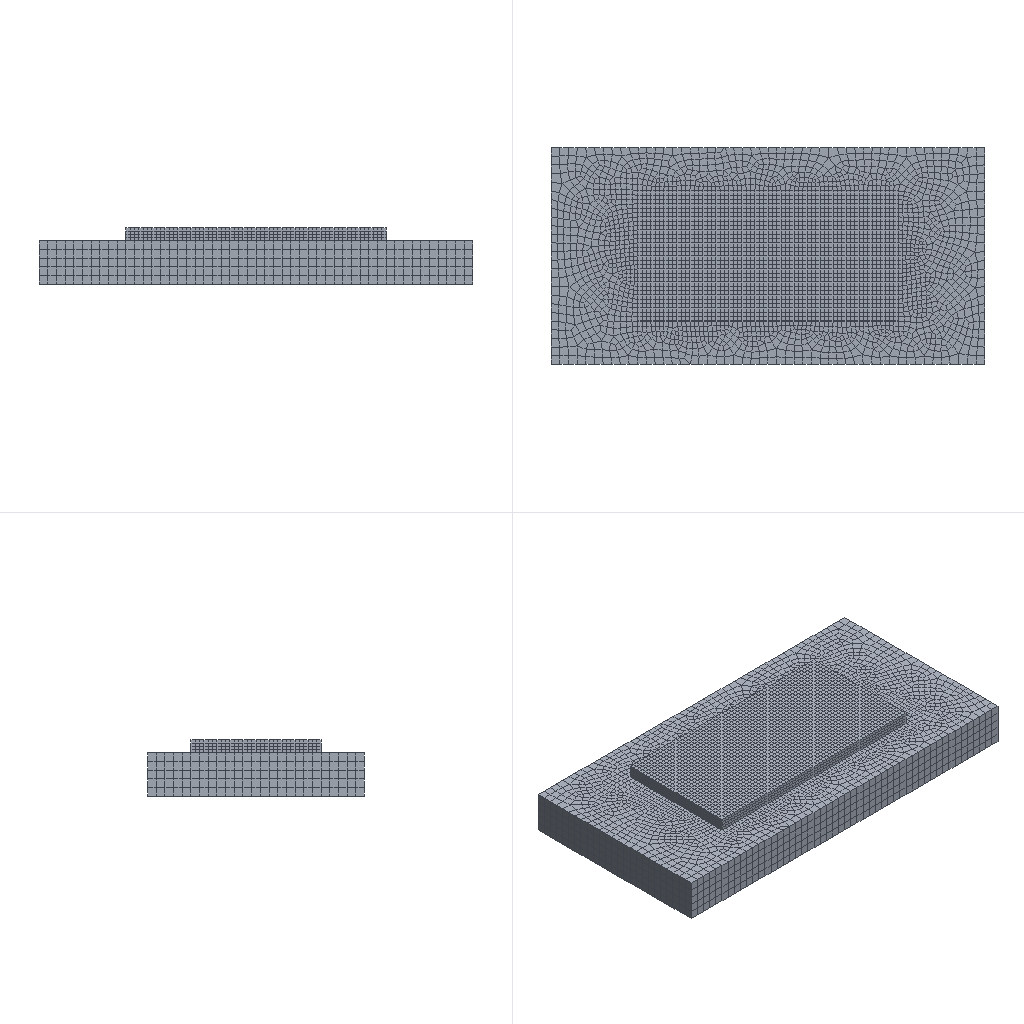Simulation study | abaqus
Set-up summary:
category,name,step,type,value,unit,region
solver,abaqus
solver,version,,,Abaqus/Standard 3DEXPERIENCE R2017x
units,not stated in the deck,,not stated
analysis,deck,,thermal,thermal
load_step,Step-1-del-all,Step-1-del-all,thermal
load_step,Step-add1,Step-add1,thermal
load_step,Step-add-l1,Step-add-l1,thermal
load_step,Step-add2,Step-add2,thermal
load_step,Step-add2-l2,Step-add2-l2,thermal
load_step,Step-add3,Step-add3,thermal
load_step,Step-add3-l3,Step-add3-l3,thermal
load_step,Step-add4,Step-add4,thermal
load_step,Step-add4-l4,Step-add4-l4,thermal
load_step,Step-add5,Step-add5,thermal
load_step,Step-add5-l5,Step-add5-l5,thermal
load_step,Step-stop1,Step-stop1,thermal
load_step,Step-add6,Step-add6,thermal
load_step,Step-add6-l6,Step-add6-l6,thermal
load_step,Step-add7,Step-add7,thermal
load_step,Step-add7-l7,Step-add7-l7,thermal
load_step,Step-add8,Step-add8,thermal
load_step,Step-add8-l8,Step-add8-l8,thermal
load_step,Step-add9,Step-add9,thermal
load_step,Step-add9-l9,Step-add9-l9,thermal
load_step,Step-add10,Step-add10,thermal
load_step,Step-add10-l10,Step-add10-l10,thermal
load_step,Step-stop2,Step-stop2,thermal
load_step,requested,,,23
mesh,nodes,,,29512
mesh,elements,,,25110
element_type,DC3D8,,solid,25110
load,load commands in deck,,count,21
bc,support commands in deck,,count,2
material,ADD,,in results
material,MATERIAL-1,,in results
check,setup vs results,,match,"per instance, exact: element labels, types and connectivity; labels of the nodes the elements use; coordinates of those nodes at SINGLE_PRECISION in 1 of 1 instance(s)"
Abaqus input file, long lists of numbers shortened:
*Heading
** Job name: Job-1 Model name: Model-1
** Generated by: Abaqus/CAE 2017
*Preprint, echo=NO, model=NO, history=NO, contact=NO
**
** PARTS
**
*Part, name=Part-1
*Node
      1,          10.,         -17.,         5.75
      2,          10.,         -17.,           5.
** (29510 more lines like these left out)
*Element, type=DC3D8
  1,   294,  2297, 12531,  1707,     1,    45,  1589,   164
  2,  2297,   300,  2002, 12531,    45,     2,    46,  1589
** (25108 more lines like these left out)
*Nset, nset=Set-1
     2,     3,     5,     6,    10,    11,    25,    26,    27,    28,    35,    36,    37,    38,    39,    40
    41,    42,    43,    44,    46,    47,    48,    49,    50,    51,    52,    53,    54,    55,    56,    57
** (1370 more lines like these left out)
*Elset, elset=Set-1, generate
  7201,  25110,      1
*Nset, nset=Set-4
     1,     2,     3,     4,     5,     6,     7,     8,     9,    10,    11,    12,    13,    14,    15,    16
    17,    18,    19,    20,    21,    22,    23,    24,    25,    26,    27,    28,    29,    30,    31,    32
** (589 more lines like these left out)
*Elset, elset=Set-4, generate
    1,  7200,     1
** Section: add
*Solid Section, elset=Set-4, material=add
,
** Section: steel
*Solid Section, elset=Set-1, material=Material-1
,
*End Part
**
**
** ASSEMBLY
**
*Assembly, name=Assembly
**
*Instance, name=Part-1-1, part=Part-1
*End Instance
**
*Nset, nset=Set-1, instance=Part-1-1
     1,     2,     3,     4,     5,     6,     7,     8,     9,    10,    11,    12,    13,    14,    15,    16
    17,    18,    19,    20,    21,    22,    23,    24,    25,    26,    27,    28,    29,    30,    31,    32
** (589 more lines like these left out)
*Elset, elset=Set-1, instance=Part-1-1, generate
    1,  7200,     1
*Nset, nset=Set-2, instance=Part-1-1
    23,    24,    25,    26,    33,    34,    35,    36,   788,   789,   790,   791,   792,   793,   794,   795
   796,   797,   798,   799,   800,   801,   802,   803,   804,   805,   806,   807,   808,   809,   810,   811
** (79 more lines like these left out)
*Elset, elset=Set-2, instance=Part-1-1, generate
 6481,  7200,     1
*Nset, nset=Set-3, instance=Part-1-1
     5,     6,     7,     8,    21,    22,    27,    28,   165,   166,   167,   168,   169,   170,   171,   172
   173,   174,   175,   176,   177,   178,   179,   180,   181,   182,   183,   184,   185,   186,   187,   188
** (79 more lines like these left out)
*Elset, elset=Set-3, instance=Part-1-1, generate
 4321,  5040,     1
*Nset, nset=Set-4, instance=Part-1-1
    21,    22,    23,    24,    25,    26,    27,    28,   709,   710,   711,   712,   713,   714,   715,   716
   717,   718,   719,   720,   721,   722,   723,   724,   725,   726,   727,   728,   729,   730,   731,   732
** (79 more lines like these left out)
*Elset, elset=Set-4, instance=Part-1-1, generate
 3601,  4320,     1
*Nset, nset=Set-5, instance=Part-1-1
     1,     2,     3,     4,     5,     6,     7,     8,    45,    46,    47,    48,    49,    50,    51,    52
    53,    54,    55,    56,    57,    58,    59,    60,    61,    62,    63,    64,    65,    66,    67,    68
** (79 more lines like these left out)
*Elset, elset=Set-5, instance=Part-1-1, generate
   1,  720,    1
*Nset, nset=Set-6, instance=Part-1-1
     1,     2,     3,     4,     9,    10,    11,    12,    45,    46,    47,    48,    49,    50,    51,    52
    53,    54,    55,    56,    57,    58,    59,    60,    61,    62,    63,    64,    65,    66,    67,    68
** (79 more lines like these left out)
*Elset, elset=Set-6, instance=Part-1-1, generate
  721,  1440,     1
*Nset, nset=Set-7, instance=Part-1-1
    23,    24,    29,    30,    31,    32,    33,    34,   788,   789,   790,   791,   792,   793,   794,   795
   796,   797,   798,   799,   800,   801,   802,   803,   804,   805,   806,   807,   808,   809,   810,   811
** (79 more lines like these left out)
*Elset, elset=Set-7, instance=Part-1-1, generate
 5041,  5760,     1
*Nset, nset=Set-8, instance=Part-1-1
    19,    20,    21,    22,    23,    24,    29,    30,   648,   649,   650,   651,   652,   653,   654,   655
   656,   657,   658,   659,   660,   661,   662,   663,   664,   665,   666,   667,   668,   669,   670,   671
** (79 more lines like these left out)
*Elset, elset=Set-8, instance=Part-1-1, generate
 5761,  6480,     1
*Nset, nset=Set-9, instance=Part-1-1
     7,     8,    17,    18,    19,    20,    21,    22,   226,   227,   228,   229,   230,   231,   232,   233
   234,   235,   236,   237,   238,   239,   240,   241,   242,   243,   244,   245,   246,   247,   248,   249
** (79 more lines like these left out)
*Elset, elset=Set-9, instance=Part-1-1, generate
 2881,  3600,     1
*Nset, nset=Set-10, instance=Part-1-1
     1,     4,     7,     8,    13,    14,    17,    18,   106,   107,   108,   109,   110,   111,   112,   113
   114,   115,   116,   117,   118,   119,   120,   121,   122,   123,   124,   125,   126,   127,   128,   129
** (79 more lines like these left out)
*Elset, elset=Set-10, instance=Part-1-1, generate
 2161,  2880,     1
*Nset, nset=Set-11, instance=Part-1-1
     1,     4,     9,    12,    13,    14,    15,    16,   106,   107,   108,   109,   110,   111,   112,   113
   114,   115,   116,   117,   118,   119,   120,   121,   122,   123,   124,   125,   126,   127,   128,   129
** (79 more lines like these left out)
*Elset, elset=Set-11, instance=Part-1-1, generate
 1441,  2160,     1
*Nset, nset=Set-12, instance=Part-1-1
    21,    22,    23,    24,    25,    26,    27,    28,   709,   710,   711,   712,   713,   714,   715,   716
   717,   718,   719,   720,   721,   722,   723,   724,   725,   726,   727,   728,   729,   730,   731,   732
** (79 more lines like these left out)
*Elset, elset=Set-12, instance=Part-1-1, generate
 3601,  4320,     1
*Nset, nset=Set-13, instance=Part-1-1, generate
     1,  29512,      1
*Elset, elset=Set-13, instance=Part-1-1, generate
     1,  25110,      1
*Nset, nset=Set-14, instance=Part-1-1, generate
     1,  29512,      1
*Elset, elset=Set-14, instance=Part-1-1, generate
     1,  25110,      1
*Nset, nset=Set-15, instance=Part-1-1, generate
     1,  29512,      1
*Elset, elset=Set-15, instance=Part-1-1, generate
     1,  25110,      1
*Elset, elset=_Surf-1_S5, internal, instance=Part-1-1
   119,   120,   239,   240,   359,   360,   479,   480,   599,   600,   719,   720,   839,   840,   959,   960
  1079,  1080,  1199,  1200,  1319,  1320,  1439,  1440,  1741,  1742,  1743,  1744,  1745,  1746,  1747,  1748
** (30 more lines like these left out)
*Elset, elset=_Surf-1_S6, internal, instance=Part-1-1
  1441,  1501,  1561,  1621,  1681,  1741,  1801,  1861,  1921,  1981,  2041,  2101,  2161,  2221,  2281,  2341
  2401,  2461,  2521,  2581,  2641,  2701,  2761,  2821,  3601,  3661,  3721,  3781,  3841,  3901,  3961,  4021
** (12 more lines like these left out)
*Elset, elset=_Surf-1_S3, internal, instance=Part-1-1
     1,     2,   121,   122,   241,   242,   361,   362,   481,   482,   601,   602,   721,   722,   841,   842
   961,   962,  1081,  1082,  1201,  1202,  1321,  1322,  2881,  2882,  3001,  3002,  3121,  3122,  3241,  3242
** (13 more lines like these left out)
*Elset, elset=_Surf-1_S4, internal, instance=Part-1-1
  1500,  1560,  1620,  1680,  1740,  1800,  1860,  1920,  1980,  2040,  2100,  2160,  2220,  2280,  2340,  2400
  2460,  2520,  2580,  2640,  2700,  2760,  2820,  2880,  2882,  2884,  2886,  2888,  2890,  2892,  2894,  2896
** (60 more lines like these left out)
*Elset, elset=_Surf-1_S2, internal, instance=Part-1-1
  1321,  1322,  1323,  1324,  1325,  1326,  1327,  1328,  1329,  1330,  1331,  1332,  1333,  1334,  1335,  1336
  1337,  1338,  1339,  1340,  1341,  1342,  1343,  1344,  1345,  1346,  1347,  1348,  1349,  1350,  1351,  1352
** (298 more lines like these left out)
*Elset, elset=_Surf-1_S1, internal, instance=Part-1-1
  5641,  5642,  5643,  5644,  5645,  5646,  5647,  5648,  5649,  5650,  5651,  5652,  5653,  5654,  5655,  5656
  5657,  5658,  5659,  5660,  5661,  5662,  5663,  5664,  5665,  5666,  5667,  5668,  5669,  5670,  5671,  5672
** (118 more lines like these left out)
*Surface, type=ELEMENT, name=Surf-1
_Surf-1_S5, S5
_Surf-1_S6, S6
_Surf-1_S4, S4
_Surf-1_S2, S2
_Surf-1_S3, S3
_Surf-1_S1, S1
*Elset, elset=_Surf-2_S5, internal, instance=Part-1-1
   119,   120,   239,   240,   359,   360,   479,   480,   599,   600,   719,   720,   839,   840,   959,   960
  1079,  1080,  1199,  1200,  1319,  1320,  1439,  1440,  1741,  1742,  1743,  1744,  1745,  1746,  1747,  1748
** (30 more lines like these left out)
*Elset, elset=_Surf-2_S6, internal, instance=Part-1-1
  1441,  1501,  1561,  1621,  1681,  1741,  1801,  1861,  1921,  1981,  2041,  2101,  2161,  2221,  2281,  2341
  2401,  2461,  2521,  2581,  2641,  2701,  2761,  2821,  3601,  3661,  3721,  3781,  3841,  3901,  3961,  4021
** (12 more lines like these left out)
*Elset, elset=_Surf-2_S3, internal, instance=Part-1-1
     1,     2,   121,   122,   241,   242,   361,   362,   481,   482,   601,   602,   721,   722,   841,   842
   961,   962,  1081,  1082,  1201,  1202,  1321,  1322,  2881,  2882,  3001,  3002,  3121,  3122,  3241,  3242
** (13 more lines like these left out)
*Elset, elset=_Surf-2_S4, internal, instance=Part-1-1
  1500,  1560,  1620,  1680,  1740,  1800,  1860,  1920,  1980,  2040,  2100,  2160,  2220,  2280,  2340,  2400
  2460,  2520,  2580,  2640,  2700,  2760,  2820,  2880,  2882,  2884,  2886,  2888,  2890,  2892,  2894,  2896
** (60 more lines like these left out)
*Elset, elset=_Surf-2_S2, internal, instance=Part-1-1
  1321,  1322,  1323,  1324,  1325,  1326,  1327,  1328,  1329,  1330,  1331,  1332,  1333,  1334,  1335,  1336
  1337,  1338,  1339,  1340,  1341,  1342,  1343,  1344,  1345,  1346,  1347,  1348,  1349,  1350,  1351,  1352
** (298 more lines like these left out)
*Elset, elset=_Surf-2_S1, internal, instance=Part-1-1
  5641,  5642,  5643,  5644,  5645,  5646,  5647,  5648,  5649,  5650,  5651,  5652,  5653,  5654,  5655,  5656
  5657,  5658,  5659,  5660,  5661,  5662,  5663,  5664,  5665,  5666,  5667,  5668,  5669,  5670,  5671,  5672
** (118 more lines like these left out)
*Surface, type=ELEMENT, name=Surf-2
_Surf-2_S5, S5
_Surf-2_S6, S6
_Surf-2_S4, S4
_Surf-2_S2, S2
_Surf-2_S3, S3
_Surf-2_S1, S1
*End Assembly
**
** MATERIALS
**
*Material, name=Material-1
*Conductivity
50.,
*Density
 7.8e-09,
*Elastic
210000., 0.3
*Plastic
300.,0.
*Specific Heat
 4.6e+08,
*Material, name=add
*Conductivity
109.,
*Density
 8.6e-09,
*Elastic
80000., 0.365
*Expansion
 1.68e-05,
*Specific Heat
 3.72e+08,
**
** PHYSICAL CONSTANTS
**
*Physical Constants, absolute zero=-273., stefan boltzmann=5.67e-08
**
** PREDEFINED FIELDS
**
** Name: Predefined Field-1   Type: Temperature
*Initial Conditions, type=TEMPERATURE
Set-14, 20.
** ----------------------------------------------------------------
**
** STEP: Step-1-del-all
**
*Step, name=Step-1-del-all, nlgeom=NO, inc=1000
*Heat Transfer, end=PERIOD, deltmx=10000.
1e-05, 1e-05, 1e-10, 1e-05,
**
** INTERACTIONS
**
** Interaction: Int-1
*Model Change, remove
Set-1,
** Interaction: Int-12
*Sradiate
Surf-1, R, 20., 0.6
** Interaction: Int-13
*Sfilm
Surf-2, F, 20., 0.1
**
** OUTPUT REQUESTS
**
*Restart, write, frequency=0
**
** FIELD OUTPUT: F-Output-1
**
*Output, field
*Node Output
NT, RFL
*Element Output, directions=YES
HFL, TEMP
*Output, history, frequency=0
*End Step
** ----------------------------------------------------------------
**
** STEP: Step-add1
**
*Step, name=Step-add1, nlgeom=NO, inc=1000
*Heat Transfer, end=PERIOD, deltmx=10000.
1e-05, 1e-05, 1e-10, 1e-05,
**
** INTERACTIONS
**
** Interaction: Int-add1
*Model Change, add
Set-2,
**
** OUTPUT REQUESTS
**
*Restart, write, frequency=0
**
** FIELD OUTPUT: F-Output-1
**
*Output, field
*Node Output
NT, RFL
*Element Output, directions=YES
HFL, TEMP
*Output, history, frequency=0
*End Step
** ----------------------------------------------------------------
**
** STEP: Step-add-l1
**
*Step, name=Step-add-l1, nlgeom=NO, inc=1000
*Heat Transfer, end=PERIOD
0.3, 3., , ,
**
** LOADS
**
** Name: Load-1   Type: Body heat flux
*Dflux, op=NEW
Set-13, BFNU, 1.
**
** OUTPUT REQUESTS
**
*Restart, write, frequency=0
**
** FIELD OUTPUT: F-Output-1
**
*Output, field
*Node Output
NT, RFL
*Element Output, directions=YES
HFL, TEMP
*Output, history, frequency=0
*End Step
** ----------------------------------------------------------------
**
** STEP: Step-add2
**
*Step, name=Step-add2, nlgeom=NO, inc=1000
*Heat Transfer, end=PERIOD, deltmx=1000.
1e-05, 1e-05, 1e-10, 1e-05,
**
** LOADS
**
** Name: Load-1   Type: Body heat flux
*Dflux, op=NEW
**
** INTERACTIONS
**
** Interaction: Int-add2
*Model Change, add
Set-12,
**
** OUTPUT REQUESTS
**
*Restart, write, frequency=0
**
** FIELD OUTPUT: F-Output-1
**
*Output, field
*Node Output
NT, RFL
*Element Output, directions=YES
HFL, TEMP
*Output, history, frequency=0
*End Step
** ----------------------------------------------------------------
**
** STEP: Step-add2-l2
**
*Step, name=Step-add2-l2, nlgeom=NO, inc=1000
*Heat Transfer, end=PERIOD
0.3, 3., , ,
**
** LOADS
**
** Name: Load-2   Type: Body heat flux
*Dflux, op=NEW
Set-15, BFNU, 1.
**
** OUTPUT REQUESTS
**
*Restart, write, frequency=0
**
** FIELD OUTPUT: F-Output-1
**
*Output, field
*Node Output
NT, RFL
*Element Output, directions=YES
HFL, TEMP
*Output, history, frequency=0
*End Step
** ----------------------------------------------------------------
**
** STEP: Step-add3
**
*Step, name=Step-add3, nlgeom=NO, inc=1000
*Heat Transfer, end=PERIOD, deltmx=10000.
1e-05, 1e-05, 3e-08, 1e-05,
**
** LOADS
**
** Name: Load-2   Type: Body heat flux
*Dflux, op=NEW
**
** INTERACTIONS
**
** Interaction: Int-add3
*Model Change, add
Set-3,
**
** OUTPUT REQUESTS
**
*Restart, write, frequency=0
**
** FIELD OUTPUT: F-Output-1
**
*Output, field
*Node Output
NT, RFL
*Element Output, directions=YES
HFL, TEMP
*Output, history, frequency=0
*End Step
** ----------------------------------------------------------------
**
** STEP: Step-add3-l3
**
*Step, name=Step-add3-l3, nlgeom=NO, inc=1000
*Heat Transfer, end=PERIOD
0.3, 3., , ,
**
** LOADS
**
** Name: Load-3   Type: Body heat flux
*Dflux, op=NEW
Set-15, BFNU, 1.
**
** OUTPUT REQUESTS
**
*Restart, write, frequency=0
**
** FIELD OUTPUT: F-Output-1
**
*Output, field
*Node Output
NT, RFL
*Element Output, directions=YES
HFL, TEMP
*Output, history, frequency=0
*End Step
** ----------------------------------------------------------------
**
** STEP: Step-add4
**
*Step, name=Step-add4, nlgeom=NO, inc=1000
*Heat Transfer, end=PERIOD, deltmx=1000.
1e-05, 1e-05, 1e-10, 1e-05,
**
** LOADS
**
** Name: Load-3   Type: Body heat flux
*Dflux, op=NEW
**
** INTERACTIONS
**
** Interaction: Int-add4
*Model Change, add
Set-5,
**
** OUTPUT REQUESTS
**
*Restart, write, frequency=0
**
** FIELD OUTPUT: F-Output-1
**
*Output, field
*Node Output
NT, RFL
*Element Output, directions=YES
HFL, TEMP
*Output, history, frequency=0
*End Step
** ----------------------------------------------------------------
**
** STEP: Step-add4-l4
**
*Step, name=Step-add4-l4, nlgeom=NO, inc=1000
*Heat Transfer, end=PERIOD
0.3, 3., , ,
**
** LOADS
**
** Name: Load-4   Type: Body heat flux
*Dflux, op=NEW
Set-15, BFNU, 1.
**
** OUTPUT REQUESTS
**
*Restart, write, frequency=0
**
** FIELD OUTPUT: F-Output-1
**
*Output, field
*Node Output
NT, RFL
*Element Output, directions=YES
HFL, TEMP
*Output, history, frequency=0
*End Step
** ----------------------------------------------------------------
**
** STEP: Step-add5
**
*Step, name=Step-add5, nlgeom=NO, inc=1000
*Heat Transfer, end=PERIOD, deltmx=1000.
1e-05, 1e-05, 1e-10, 1e-05,
**
** LOADS
**
** Name: Load-4   Type: Body heat flux
*Dflux, op=NEW
**
** INTERACTIONS
**
** Interaction: Int-add5
*Model Change, add
Set-6,
**
** OUTPUT REQUESTS
**
*Restart, write, frequency=0
**
** FIELD OUTPUT: F-Output-1
**
*Output, field
*Node Output
NT, RFL
*Element Output, directions=YES
HFL, TEMP
*Output, history, frequency=0
*End Step
** ----------------------------------------------------------------
**
** STEP: Step-add5-l5
**
*Step, name=Step-add5-l5, nlgeom=NO, inc=1000
*Heat Transfer, end=PERIOD
0.3, 3., , ,
**
** LOADS
**
** Name: Load-5   Type: Body heat flux
*Dflux, op=NEW
Set-15, BFNU, 1.
**
** OUTPUT REQUESTS
**
*Restart, write, frequency=0
**
** FIELD OUTPUT: F-Output-1
**
*Output, field
*Node Output
NT, RFL
*Element Output, directions=YES
HFL, TEMP
*Output, history, frequency=0
*End Step
** ----------------------------------------------------------------
**
** STEP: Step-stop1
**
*Step, name=Step-stop1, nlgeom=NO, inc=1000
*Heat Transfer, end=PERIOD
0.3, 15., , ,
**
** LOADS
**
** Name: Load-5   Type: Body heat flux
*Dflux, op=NEW
** Name: Load-stop   Type: Body heat flux
*Dflux, op=NEW
Set-15, BFNU, 1.
**
** OUTPUT REQUESTS
**
*Restart, write, frequency=0
**
** FIELD OUTPUT: F-Output-1
**
*Output, field
*Node Output
NT, RFL
*Element Output, directions=YES
HFL, TEMP
*Output, history, frequency=0
*End Step
** ----------------------------------------------------------------
**
** STEP: Step-add6
**
*Step, name=Step-add6, nlgeom=NO, inc=1000
*Heat Transfer, end=PERIOD, deltmx=1000.
1e-05, 1e-05, 1e-10, 1e-05,
**
** LOADS
**
** Name: Load-stop   Type: Body heat flux
*Dflux, op=NEW
**
** INTERACTIONS
**
** Interaction: Int-add6
*Model Change, add
Set-7,
**
** OUTPUT REQUESTS
**
*Restart, write, frequency=0
**
** FIELD OUTPUT: F-Output-1
**
*Output, field
*Node Output
NT, RFL
*Element Output, directions=YES
HFL, TEMP
*Output, history, frequency=0
*End Step
** ----------------------------------------------------------------
**
** STEP: Step-add6-l6
**
*Step, name=Step-add6-l6, nlgeom=NO, inc=1000
*Heat Transfer, end=PERIOD
0.3, 3., , ,
**
** LOADS
**
** Name: Load-6   Type: Body heat flux
*Dflux, op=NEW
Set-15, BFNU, 1.
**
** OUTPUT REQUESTS
**
*Restart, write, frequency=0
**
** FIELD OUTPUT: F-Output-1
**
*Output, field
*Node Output
NT, RFL
*Element Output, directions=YES
HFL, TEMP
*Output, history, frequency=0
*End Step
** ----------------------------------------------------------------
**
** STEP: Step-add7
**
*Step, name=Step-add7, nlgeom=NO, inc=1000
*Heat Transfer, end=PERIOD, deltmx=10000.
1e-05, 1e-05, 1e-10, 1e-05,
**
** LOADS
**
** Name: Load-6   Type: Body heat flux
*Dflux, op=NEW
**
** INTERACTIONS
**
** Interaction: Int-add7
*Model Change, add
Set-8,
**
** OUTPUT REQUESTS
**
*Restart, write, frequency=0
**
** FIELD OUTPUT: F-Output-1
**
*Output, field
*Node Output
NT, RFL
*Element Output, directions=YES
HFL, TEMP
*Output, history, frequency=0
*End Step
** ----------------------------------------------------------------
**
** STEP: Step-add7-l7
**
*Step, name=Step-add7-l7, nlgeom=NO, inc=1000
*Heat Transfer, end=PERIOD
0.3, 3., , ,
**
** LOADS
**
** Name: Load-7   Type: Body heat flux
*Dflux, op=NEW
Set-15, BFNU, 1.
**
** OUTPUT REQUESTS
**
*Restart, write, frequency=0
**
** FIELD OUTPUT: F-Output-1
**
*Output, field
*Node Output
NT, RFL
*Element Output, directions=YES
HFL, TEMP
*Output, history, frequency=0
*End Step
** ----------------------------------------------------------------
**
** STEP: Step-add8
**
*Step, name=Step-add8, nlgeom=NO, inc=1000
*Heat Transfer, end=PERIOD, deltmx=1000.
1e-05, 1e-05, 1e-10, 1e-05,
**
** LOADS
**
** Name: Load-7   Type: Body heat flux
*Dflux, op=NEW
Set-15, BFNU, 1.
**
** INTERACTIONS
**
** Interaction: Int-add8
*Model Change, add
Set-9,
**
** OUTPUT REQUESTS
**
*Restart, write, frequency=0
**
** FIELD OUTPUT: F-Output-1
**
*Output, field
*Node Output
NT, RFL
*Element Output, directions=YES
HFL, TEMP
*Output, history, frequency=0
*End Step
** ----------------------------------------------------------------
**
** STEP: Step-add8-l8
**
*Step, name=Step-add8-l8, nlgeom=NO, inc=1000
*Heat Transfer, end=PERIOD
0.3, 3., , ,
**
** LOADS
**
** Name: Load-7   Type: Body heat flux
*Dflux, op=NEW
Set-15, BFNU, 1.
** Name: Load-8   Type: Body heat flux
*Dflux, op=NEW
Set-15, BFNU, 1.
**
** OUTPUT REQUESTS
**
*Restart, write, frequency=0
**
** FIELD OUTPUT: F-Output-1
**
*Output, field
*Node Output
NT, RFL
*Element Output, directions=YES
HFL, TEMP
*Output, history, frequency=0
*End Step
** ----------------------------------------------------------------
**
** STEP: Step-add9
**
*Step, name=Step-add9, nlgeom=NO, inc=1000
*Heat Transfer, end=PERIOD, deltmx=10000.
1e-05, 1e-05, 1e-10, 1e-05,
**
** LOADS
**
** Name: Load-7   Type: Body heat flux
*Dflux, op=NEW
Set-15, BFNU, 1.
** Name: Load-8   Type: Body heat flux
*Dflux, op=NEW
**
** INTERACTIONS
**
** Interaction: Int-add9
*Model Change, add
Set-10,
**
** OUTPUT REQUESTS
**
*Restart, write, frequency=0
**
** FIELD OUTPUT: F-Output-1
**
*Output, field
*Node Output
NT, RFL
*Element Output, directions=YES
HFL, TEMP
*Output, history, frequency=0
*End Step
** ----------------------------------------------------------------
**
** STEP: Step-add9-l9
**
*Step, name=Step-add9-l9, nlgeom=NO, inc=1000
*Heat Transfer, end=PERIOD
0.3, 3., , ,
**
** LOADS
**
** Name: Load-7   Type: Body heat flux
*Dflux, op=NEW
Set-15, BFNU, 1.
** Name: Load-9   Type: Body heat flux
*Dflux, op=NEW
Set-15, BFNU, 1.
**
** OUTPUT REQUESTS
**
*Restart, write, frequency=0
**
** FIELD OUTPUT: F-Output-1
**
*Output, field
*Node Output
NT, RFL
*Element Output, directions=YES
HFL, TEMP
*Output, history, frequency=0
*End Step
** ----------------------------------------------------------------
**
** STEP: Step-add10
**
*Step, name=Step-add10, nlgeom=NO, inc=1000
*Heat Transfer, end=PERIOD, deltmx=10000.
1e-05, 1e-05, 1e-10, 1e-05,
**
** LOADS
**
** Name: Load-7   Type: Body heat flux
*Dflux, op=NEW
Set-15, BFNU, 1.
** Name: Load-9   Type: Body heat flux
*Dflux, op=NEW
**
** INTERACTIONS
**
** Interaction: Int-add10
*Model Change, add
Set-11,
**
** OUTPUT REQUESTS
**
*Restart, write, frequency=0
**
** FIELD OUTPUT: F-Output-1
**
*Output, field
*Node Output
NT, RFL
*Element Output, directions=YES
HFL, TEMP
*Output, history, frequency=0
*End Step
** ----------------------------------------------------------------
**
** STEP: Step-add10-l10
**
*Step, name=Step-add10-l10, nlgeom=NO, inc=1000
*Heat Transfer, end=PERIOD
0.3, 3., , ,
**
** LOADS
**
** Name: Load-7   Type: Body heat flux
*Dflux, op=NEW
Set-15, BFNU, 1.
** Name: Load-10   Type: Body heat flux
*Dflux, op=NEW
Set-15, BFNU, 1.
**
** OUTPUT REQUESTS
**
*Restart, write, frequency=0
**
** FIELD OUTPUT: F-Output-1
**
*Output, field
*Node Output
NT, RFL
*Element Output, directions=YES
HFL, TEMP
*Output, history, frequency=0
*End Step
** ----------------------------------------------------------------
**
** STEP: Step-stop2
**
*Step, name=Step-stop2, nlgeom=NO, inc=1000
*Heat Transfer, end=PERIOD
0.3, 15., , ,
**
** LOADS
**
** Name: Load-7   Type: Body heat flux
*Dflux, op=NEW
Set-15, BFNU, 1.
** Name: Load-10   Type: Body heat flux
*Dflux, op=NEW
** Name: Load-stop2   Type: Body heat flux
*Dflux, op=NEW
Set-15, BFNU, 1.
**
** OUTPUT REQUESTS
**
*Restart, write, frequency=0
**
** FIELD OUTPUT: F-Output-1
**
*Output, field
*Node Output
NT, RFL
*Element Output, directions=YES
HFL, TEMP
*Output, history, frequency=0
*End Step
Results summary:
result,step,,partial,increments=0 time=0.0/1e-05
result,step,,partial,increments=0 time=0.0/1e-05
result,step,,partial,increments=0 time=0.0/3.0
result,step,,partial,increments=0 time=0.0/1e-05
result,step,,partial,increments=0 time=0.0/3.0
result,step,,partial,increments=0 time=0.0/1e-05
result,step,,partial,increments=0 time=0.0/3.0
result,step,,partial,increments=0 time=0.0/1e-05
result,step,,partial,increments=0 time=0.0/3.0
result,step,,partial,increments=0 time=0.0/1e-05
result,step,,partial,increments=0 time=0.0/3.0
result,step,,partial,increments=0 time=0.0/15.0
result,step,,partial,increments=0 time=0.0/1e-05
result,step,,partial,increments=0 time=0.0/3.0
result,step,,partial,increments=0 time=0.0/1e-05
result,step,,partial,increments=0 time=0.0/3.0
result,step,,partial,increments=0 time=0.0/1e-05
result,step,,partial,increments=0 time=0.0/3.0
result,step,,partial,increments=0 time=0.0/1e-05
result,step,,partial,increments=0 time=0.0/3.0
result,step,,partial,increments=0 time=0.0/1e-05
result,step,,partial,increments=0 time=0.0/3.0
result,step,,partial,increments=0 time=0.0/15.0
result,analysis,,,thermal
result,last_loadstep,,,23
result,primary field,,,NT11